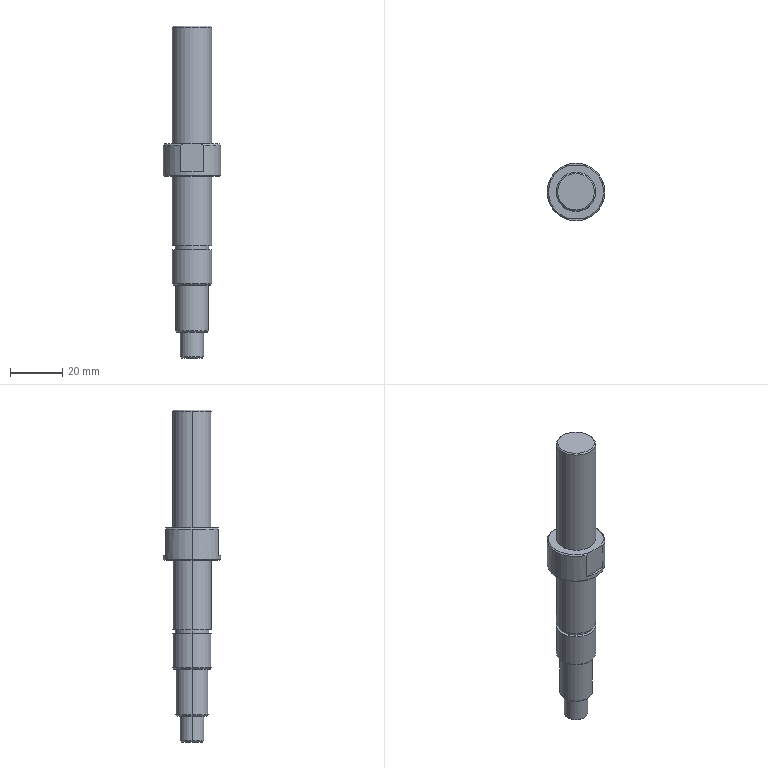Part | STEP file | 10000020499swp000-1 | 1 solid | 43 faces | box 22 x 22 x 126.85 mm | volume 22513 mm3 | cylinder 16 | cone 15 | plane 12 | commonest cylinder face diameters 15 x6 3.3 x2 9 x2 12.5 x2 12.8 x2 22 x2
STEP:
#1=CARTESIAN_POINT('',(7.5,0.,-84.));
#2=VERTEX_POINT('',#1);
#3=CARTESIAN_POINT('',(-7.5,0.,-84.));
#4=VERTEX_POINT('',#3);
#5=CARTESIAN_POINT('',(0.,0.,-84.));
#6=DIRECTION('',(0.,0.,1.));
#7=DIRECTION('',(1.,0.,0.));
#8=AXIS2_PLACEMENT_3D('',#5,#6,#7);
#9=CIRCLE('',#8,7.5);
#10=EDGE_CURVE('',#2,#4,#9,.T.);
#11=ORIENTED_EDGE('',*,*,#10,.T.);
#12=CARTESIAN_POINT('',(-7.5,0.,-57.5));
#13=VERTEX_POINT('',#12);
#14=CARTESIAN_POINT('',(-7.5,0.,-99.));
#15=DIRECTION('',(0.,0.,1.));
#16=VECTOR('',#15,1000.);
#17=LINE('',#14,#16);
#18=EDGE_CURVE('',#4,#13,#17,.T.);
#19=ORIENTED_EDGE('',*,*,#18,.T.);
#20=CARTESIAN_POINT('',(7.5,0.,-57.5));
#21=VERTEX_POINT('',#20);
#22=CARTESIAN_POINT('',(0.,0.,-57.5));
#23=DIRECTION('',(0.,0.,-1.));
#24=DIRECTION('',(-1.,0.,0.));
#25=AXIS2_PLACEMENT_3D('',#22,#23,#24);
#26=CIRCLE('',#25,7.5);
#27=EDGE_CURVE('',#13,#21,#26,.T.);
#28=ORIENTED_EDGE('',*,*,#27,.T.);
#29=CARTESIAN_POINT('',(7.5,0.,-99.));
#30=DIRECTION('',(0.,0.,1.));
#31=VECTOR('',#30,1000.);
#32=LINE('',#29,#31);
#33=EDGE_CURVE('',#2,#21,#32,.T.);
#34=ORIENTED_EDGE('',*,*,#33,.F.);
#35=EDGE_LOOP('',(#11,#19,#28,#34));
#36=FACE_OUTER_BOUND('',#35,.T.);
#37=CARTESIAN_POINT('',(0.,0.,-99.));
#38=DIRECTION('',(0.,0.,1.));
#39=DIRECTION('',(1.,0.,0.));
#40=AXIS2_PLACEMENT_3D('',#37,#38,#39);
#41=CYLINDRICAL_SURFACE('',#40,7.5);
#42=ADVANCED_FACE('',(#36),#41,.T.);
#43=CARTESIAN_POINT('',(-10.5,0.,-57.5));
#44=VERTEX_POINT('',#43);
#45=CARTESIAN_POINT('',(10.5,0.,-57.5));
#46=VERTEX_POINT('',#45);
#47=CARTESIAN_POINT('',(0.,0.,-57.5));
#48=DIRECTION('',(0.,0.,-1.));
#49=DIRECTION('',(-1.,0.,0.));
#50=AXIS2_PLACEMENT_3D('',#47,#48,#49);
#51=CIRCLE('',#50,10.5);
#52=EDGE_CURVE('',#44,#46,#51,.T.);
#53=ORIENTED_EDGE('',*,*,#52,.F.);
#54=CARTESIAN_POINT('',(-11.,0.,-57.));
#55=VERTEX_POINT('',#54);
#56=CARTESIAN_POINT('',(-10.5,0.,-57.5));
#57=DIRECTION('',(-0.7071,0.,0.7071));
#58=VECTOR('',#57,1000.);
#59=LINE('',#56,#58);
#60=EDGE_CURVE('',#44,#55,#59,.T.);
#61=ORIENTED_EDGE('',*,*,#60,.T.);
#62=CARTESIAN_POINT('',(11.,0.,-57.));
#63=VERTEX_POINT('',#62);
#64=CARTESIAN_POINT('',(0.,0.,-57.));
#65=DIRECTION('',(0.,0.,1.));
#66=DIRECTION('',(-1.,0.,0.));
#67=AXIS2_PLACEMENT_3D('',#64,#65,#66);
#68=CIRCLE('',#67,11.);
#69=EDGE_CURVE('',#63,#55,#68,.T.);
#70=ORIENTED_EDGE('',*,*,#69,.F.);
#71=CARTESIAN_POINT('',(10.5,0.,-57.5));
#72=DIRECTION('',(0.7071,0.,0.7071));
#73=VECTOR('',#72,1000.);
#74=LINE('',#71,#73);
#75=EDGE_CURVE('',#46,#63,#74,.T.);
#76=ORIENTED_EDGE('',*,*,#75,.F.);
#77=EDGE_LOOP('',(#53,#61,#70,#76));
#78=FACE_OUTER_BOUND('',#77,.T.);
#79=CARTESIAN_POINT('',(0.,0.,-57.5));
#80=DIRECTION('',(0.,0.,1.));
#81=DIRECTION('',(1.,0.,0.));
#82=AXIS2_PLACEMENT_3D('',#79,#80,#81);
#83=CONICAL_SURFACE('',#82,10.5,0.7854);
#84=ADVANCED_FACE('',(#78),#83,.T.);
#85=ORIENTED_EDGE('',*,*,#69,.T.);
#86=CARTESIAN_POINT('',(-11.,0.,-45.5));
#87=VERTEX_POINT('',#86);
#88=CARTESIAN_POINT('',(-11.,0.,-57.5));
#89=DIRECTION('',(0.,0.,1.));
#90=VECTOR('',#89,1000.);
#91=LINE('',#88,#90);
#92=EDGE_CURVE('',#55,#87,#91,.T.);
#93=ORIENTED_EDGE('',*,*,#92,.T.);
#94=CARTESIAN_POINT('',(-4.583,10.,-45.5));
#95=VERTEX_POINT('',#94);
#96=CARTESIAN_POINT('',(0.,0.,-45.5));
#97=DIRECTION('',(0.,0.,-1.));
#98=DIRECTION('',(-1.,0.,0.));
#99=AXIS2_PLACEMENT_3D('',#96,#97,#98);
#100=CIRCLE('',#99,11.);
#101=EDGE_CURVE('',#87,#95,#100,.T.);
#102=ORIENTED_EDGE('',*,*,#101,.T.);
#103=CARTESIAN_POINT('',(-4.583,10.,-55.5));
#104=VERTEX_POINT('',#103);
#105=CARTESIAN_POINT('',(-4.583,10.,-57.5));
#106=DIRECTION('',(0.,0.,1.));
#107=VECTOR('',#106,1000.);
#108=LINE('',#105,#107);
#109=EDGE_CURVE('',#104,#95,#108,.T.);
#110=ORIENTED_EDGE('',*,*,#109,.F.);
#111=CARTESIAN_POINT('',(4.583,10.,-55.5));
#112=VERTEX_POINT('',#111);
#113=CARTESIAN_POINT('',(0.,0.,-55.5));
#114=DIRECTION('',(0.,0.,1.));
#115=DIRECTION('',(1.,0.,0.));
#116=AXIS2_PLACEMENT_3D('',#113,#114,#115);
#117=CIRCLE('',#116,11.);
#118=EDGE_CURVE('',#112,#104,#117,.T.);
#119=ORIENTED_EDGE('',*,*,#118,.F.);
#120=CARTESIAN_POINT('',(4.583,10.,-45.5));
#121=VERTEX_POINT('',#120);
#122=CARTESIAN_POINT('',(4.583,10.,-57.5));
#123=DIRECTION('',(0.,0.,-1.));
#124=VECTOR('',#123,1000.);
#125=LINE('',#122,#124);
#126=EDGE_CURVE('',#121,#112,#125,.T.);
#127=ORIENTED_EDGE('',*,*,#126,.F.);
#128=CARTESIAN_POINT('',(11.,0.,-45.5));
#129=VERTEX_POINT('',#128);
#130=CARTESIAN_POINT('',(0.,0.,-45.5));
#131=DIRECTION('',(0.,0.,-1.));
#132=DIRECTION('',(-1.,0.,0.));
#133=AXIS2_PLACEMENT_3D('',#130,#131,#132);
#134=CIRCLE('',#133,11.);
#135=EDGE_CURVE('',#121,#129,#134,.T.);
#136=ORIENTED_EDGE('',*,*,#135,.T.);
#137=CARTESIAN_POINT('',(11.,0.,-57.5));
#138=DIRECTION('',(0.,0.,1.));
#139=VECTOR('',#138,1000.);
#140=LINE('',#137,#139);
#141=EDGE_CURVE('',#63,#129,#140,.T.);
#142=ORIENTED_EDGE('',*,*,#141,.F.);
#143=EDGE_LOOP('',(#85,#93,#102,#110,#119,#127,#136,#142));
#144=FACE_OUTER_BOUND('',#143,.T.);
#145=CARTESIAN_POINT('',(0.,0.,-57.5));
#146=DIRECTION('',(0.,0.,1.));
#147=DIRECTION('',(1.,0.,0.));
#148=AXIS2_PLACEMENT_3D('',#145,#146,#147);
#149=CYLINDRICAL_SURFACE('',#148,11.);
#150=ADVANCED_FACE('',(#144),#149,.T.);
#151=CARTESIAN_POINT('',(-10.5,0.,-45.));
#152=VERTEX_POINT('',#151);
#153=CARTESIAN_POINT('',(-3.202,-10.,-45.));
#154=VERTEX_POINT('',#153);
#155=CARTESIAN_POINT('',(0.,0.,-45.));
#156=DIRECTION('',(0.,0.,1.));
#157=DIRECTION('',(-1.,0.,0.));
#158=AXIS2_PLACEMENT_3D('',#155,#156,#157);
#159=CIRCLE('',#158,10.5);
#160=EDGE_CURVE('',#152,#154,#159,.T.);
#161=ORIENTED_EDGE('',*,*,#160,.F.);
#162=CARTESIAN_POINT('',(-11.,0.,-45.5));
#163=DIRECTION('',(-0.7071,0.,-0.7071));
#164=VECTOR('',#163,1000.);
#165=LINE('',#162,#164);
#166=EDGE_CURVE('',#152,#87,#165,.T.);
#167=ORIENTED_EDGE('',*,*,#166,.T.);
#168=CARTESIAN_POINT('',(-4.583,-10.,-45.5));
#169=VERTEX_POINT('',#168);
#170=CARTESIAN_POINT('',(0.,0.,-45.5));
#171=DIRECTION('',(0.,0.,-1.));
#172=DIRECTION('',(-1.,0.,0.));
#173=AXIS2_PLACEMENT_3D('',#170,#171,#172);
#174=CIRCLE('',#173,11.);
#175=EDGE_CURVE('',#169,#87,#174,.T.);
#176=ORIENTED_EDGE('',*,*,#175,.F.);
#177=CARTESIAN_POINT('',(-4.583,-10.,-45.5));
#178=CARTESIAN_POINT('',(-4.131,-10.,-45.312));
#179=CARTESIAN_POINT('',(-3.672,-10.,-45.143));
#180=CARTESIAN_POINT('',(-3.202,-10.,-45.));
#181=B_SPLINE_CURVE_WITH_KNOTS('',3,(#177,#178,#179,#180),.UNSPECIFIED.,.F.,.F.,(4,4),(0.02198,0.02345),.UNSPECIFIED.);
#182=EDGE_CURVE('',#169,#154,#181,.T.);
#183=ORIENTED_EDGE('',*,*,#182,.T.);
#184=EDGE_LOOP('',(#161,#167,#176,#183));
#185=FACE_OUTER_BOUND('',#184,.T.);
#186=CARTESIAN_POINT('',(0.,0.,-45.5));
#187=DIRECTION('',(0.,0.,-1.));
#188=DIRECTION('',(-1.,0.,0.));
#189=AXIS2_PLACEMENT_3D('',#186,#187,#188);
#190=CONICAL_SURFACE('',#189,11.,0.7854);
#191=ADVANCED_FACE('',(#185),#190,.T.);
#192=CARTESIAN_POINT('',(7.5,0.,-45.));
#193=VERTEX_POINT('',#192);
#194=CARTESIAN_POINT('',(-7.5,0.,-45.));
#195=VERTEX_POINT('',#194);
#196=CARTESIAN_POINT('',(0.,0.,-45.));
#197=DIRECTION('',(0.,0.,1.));
#198=DIRECTION('',(-1.,0.,0.));
#199=AXIS2_PLACEMENT_3D('',#196,#197,#198);
#200=CIRCLE('',#199,7.5);
#201=EDGE_CURVE('',#193,#195,#200,.T.);
#202=ORIENTED_EDGE('',*,*,#201,.T.);
#203=CARTESIAN_POINT('',(-7.5,0.,-0.5));
#204=VERTEX_POINT('',#203);
#205=CARTESIAN_POINT('',(-7.5,0.,-45.));
#206=DIRECTION('',(0.,0.,1.));
#207=VECTOR('',#206,1000.);
#208=LINE('',#205,#207);
#209=EDGE_CURVE('',#195,#204,#208,.T.);
#210=ORIENTED_EDGE('',*,*,#209,.T.);
#211=CARTESIAN_POINT('',(7.5,0.,-0.5));
#212=VERTEX_POINT('',#211);
#213=CARTESIAN_POINT('',(0.,0.,-0.5));
#214=DIRECTION('',(0.,0.,-1.));
#215=DIRECTION('',(1.,0.,0.));
#216=AXIS2_PLACEMENT_3D('',#213,#214,#215);
#217=CIRCLE('',#216,7.5);
#218=EDGE_CURVE('',#204,#212,#217,.T.);
#219=ORIENTED_EDGE('',*,*,#218,.T.);
#220=CARTESIAN_POINT('',(7.5,0.,-45.));
#221=DIRECTION('',(0.,0.,1.));
#222=VECTOR('',#221,1000.);
#223=LINE('',#220,#222);
#224=EDGE_CURVE('',#193,#212,#223,.T.);
#225=ORIENTED_EDGE('',*,*,#224,.F.);
#226=EDGE_LOOP('',(#202,#210,#219,#225));
#227=FACE_OUTER_BOUND('',#226,.T.);
#228=CARTESIAN_POINT('',(0.,0.,-45.));
#229=DIRECTION('',(0.,0.,1.));
#230=DIRECTION('',(1.,0.,0.));
#231=AXIS2_PLACEMENT_3D('',#228,#229,#230);
#232=CYLINDRICAL_SURFACE('',#231,7.5);
#233=ADVANCED_FACE('',(#227),#232,.T.);
#234=CARTESIAN_POINT('',(7.,0.,0.));
#235=VERTEX_POINT('',#234);
#236=CARTESIAN_POINT('',(-7.,0.,0.));
#237=VERTEX_POINT('',#236);
#238=CARTESIAN_POINT('',(0.,0.,0.));
#239=DIRECTION('',(0.,0.,1.));
#240=DIRECTION('',(1.,0.,0.));
#241=AXIS2_PLACEMENT_3D('',#238,#239,#240);
#242=CIRCLE('',#241,7.);
#243=EDGE_CURVE('',#235,#237,#242,.T.);
#244=ORIENTED_EDGE('',*,*,#243,.F.);
#245=CARTESIAN_POINT('',(7.,0.,0.));
#246=DIRECTION('',(0.7071,0.,-0.7071));
#247=VECTOR('',#246,1000.);
#248=LINE('',#245,#247);
#249=EDGE_CURVE('',#235,#212,#248,.T.);
#250=ORIENTED_EDGE('',*,*,#249,.T.);
#251=ORIENTED_EDGE('',*,*,#218,.F.);
#252=CARTESIAN_POINT('',(-7.,0.,0.));
#253=DIRECTION('',(-0.7071,0.,-0.7071));
#254=VECTOR('',#253,1000.);
#255=LINE('',#252,#254);
#256=EDGE_CURVE('',#237,#204,#255,.T.);
#257=ORIENTED_EDGE('',*,*,#256,.F.);
#258=EDGE_LOOP('',(#244,#250,#251,#257));
#259=FACE_OUTER_BOUND('',#258,.T.);
#260=CARTESIAN_POINT('',(0.,0.,0.));
#261=DIRECTION('',(0.,0.,-1.));
#262=DIRECTION('',(-1.,0.,0.));
#263=AXIS2_PLACEMENT_3D('',#260,#261,#262);
#264=CONICAL_SURFACE('',#263,7.,0.7854);
#265=ADVANCED_FACE('',(#259),#264,.T.);
#266=CARTESIAN_POINT('',(6.4,0.,-85.5));
#267=VERTEX_POINT('',#266);
#268=CARTESIAN_POINT('',(-6.4,0.,-85.5));
#269=VERTEX_POINT('',#268);
#270=CARTESIAN_POINT('',(0.,0.,-85.5));
#271=DIRECTION('',(0.,0.,1.));
#272=DIRECTION('',(1.,0.,0.));
#273=AXIS2_PLACEMENT_3D('',#270,#271,#272);
#274=CIRCLE('',#273,6.4);
#275=EDGE_CURVE('',#267,#269,#274,.T.);
#276=ORIENTED_EDGE('',*,*,#275,.T.);
#277=CARTESIAN_POINT('',(-6.4,0.,-84.));
#278=VERTEX_POINT('',#277);
#279=CARTESIAN_POINT('',(-6.4,0.,-126.85));
#280=DIRECTION('',(0.,0.,1.));
#281=VECTOR('',#280,1000.);
#282=LINE('',#279,#281);
#283=EDGE_CURVE('',#269,#278,#282,.T.);
#284=ORIENTED_EDGE('',*,*,#283,.T.);
#285=CARTESIAN_POINT('',(6.4,0.,-84.));
#286=VERTEX_POINT('',#285);
#287=CARTESIAN_POINT('',(0.,0.,-84.));
#288=DIRECTION('',(0.,0.,1.));
#289=DIRECTION('',(1.,0.,0.));
#290=AXIS2_PLACEMENT_3D('',#287,#288,#289);
#291=CIRCLE('',#290,6.4);
#292=EDGE_CURVE('',#286,#278,#291,.T.);
#293=ORIENTED_EDGE('',*,*,#292,.F.);
#294=CARTESIAN_POINT('',(6.4,0.,-126.85));
#295=DIRECTION('',(0.,0.,1.));
#296=VECTOR('',#295,1000.);
#297=LINE('',#294,#296);
#298=EDGE_CURVE('',#267,#286,#297,.T.);
#299=ORIENTED_EDGE('',*,*,#298,.F.);
#300=EDGE_LOOP('',(#276,#284,#293,#299));
#301=FACE_OUTER_BOUND('',#300,.T.);
#302=CARTESIAN_POINT('',(0.,0.,-126.85));
#303=DIRECTION('',(0.,0.,1.));
#304=DIRECTION('',(1.,0.,0.));
#305=AXIS2_PLACEMENT_3D('',#302,#303,#304);
#306=CYLINDRICAL_SURFACE('',#305,6.4);
#307=ADVANCED_FACE('',(#301),#306,.T.);
#308=CARTESIAN_POINT('',(1.65,0.,-112.75));
#309=VERTEX_POINT('',#308);
#310=CARTESIAN_POINT('',(-1.65,0.,-112.75));
#311=VERTEX_POINT('',#310);
#312=CARTESIAN_POINT('',(0.,0.,-112.75));
#313=DIRECTION('',(0.,0.,-1.));
#314=DIRECTION('',(-1.,0.,0.));
#315=AXIS2_PLACEMENT_3D('',#312,#313,#314);
#316=CIRCLE('',#315,1.65);
#317=EDGE_CURVE('',#309,#311,#316,.T.);
#318=ORIENTED_EDGE('',*,*,#317,.F.);
#319=CARTESIAN_POINT('',(1.65,0.,-126.85));
#320=VERTEX_POINT('',#319);
#321=CARTESIAN_POINT('',(1.65,0.,-126.85));
#322=DIRECTION('',(0.,0.,-1.));
#323=VECTOR('',#322,1000.);
#324=LINE('',#321,#323);
#325=EDGE_CURVE('',#309,#320,#324,.T.);
#326=ORIENTED_EDGE('',*,*,#325,.T.);
#327=CARTESIAN_POINT('',(-1.65,0.,-126.85));
#328=VERTEX_POINT('',#327);
#329=CARTESIAN_POINT('',(0.,0.,-126.85));
#330=DIRECTION('',(0.,0.,-1.));
#331=DIRECTION('',(-1.,0.,0.));
#332=AXIS2_PLACEMENT_3D('',#329,#330,#331);
#333=CIRCLE('',#332,1.65);
#334=EDGE_CURVE('',#320,#328,#333,.T.);
#335=ORIENTED_EDGE('',*,*,#334,.T.);
#336=CARTESIAN_POINT('',(-1.65,0.,-126.85));
#337=DIRECTION('',(0.,0.,-1.));
#338=VECTOR('',#337,1000.);
#339=LINE('',#336,#338);
#340=EDGE_CURVE('',#311,#328,#339,.T.);
#341=ORIENTED_EDGE('',*,*,#340,.F.);
#342=EDGE_LOOP('',(#318,#326,#335,#341));
#343=FACE_OUTER_BOUND('',#342,.T.);
#344=CARTESIAN_POINT('',(0.,0.,-126.85));
#345=DIRECTION('',(0.,0.,-1.));
#346=DIRECTION('',(-1.,0.,0.));
#347=AXIS2_PLACEMENT_3D('',#344,#345,#346);
#348=CYLINDRICAL_SURFACE('',#347,1.65);
#349=ADVANCED_FACE('',(#343),#348,.F.);
#350=CARTESIAN_POINT('',(0.,0.,-111.759));
#351=VERTEX_POINT('',#350);
#352=CARTESIAN_POINT('',(-1.65,0.,-112.75));
#353=DIRECTION('',(-0.8572,0.,-0.515));
#354=VECTOR('',#353,1000.);
#355=LINE('',#352,#354);
#356=EDGE_CURVE('',#351,#311,#355,.T.);
#357=ORIENTED_EDGE('',*,*,#356,.F.);
#358=CARTESIAN_POINT('',(1.65,0.,-112.75));
#359=DIRECTION('',(0.8572,0.,-0.515));
#360=VECTOR('',#359,1000.);
#361=LINE('',#358,#360);
#362=EDGE_CURVE('',#351,#309,#361,.T.);
#363=ORIENTED_EDGE('',*,*,#362,.T.);
#364=ORIENTED_EDGE('',*,*,#317,.T.);
#365=EDGE_LOOP('',(#357,#363,#364));
#366=FACE_OUTER_BOUND('',#365,.T.);
#367=CARTESIAN_POINT('',(0.,0.,-112.75));
#368=DIRECTION('',(0.,0.,-1.));
#369=DIRECTION('',(-1.,0.,0.));
#370=AXIS2_PLACEMENT_3D('',#367,#368,#369);
#371=CONICAL_SURFACE('',#370,1.65,1.03);
#372=ADVANCED_FACE('',(#366),#371,.F.);
#373=CARTESIAN_POINT('',(-4.,0.,-126.85));
#374=VERTEX_POINT('',#373);
#375=CARTESIAN_POINT('',(4.,0.,-126.85));
#376=VERTEX_POINT('',#375);
#377=CARTESIAN_POINT('',(0.,0.,-126.85));
#378=DIRECTION('',(0.,0.,-1.));
#379=DIRECTION('',(-1.,0.,0.));
#380=AXIS2_PLACEMENT_3D('',#377,#378,#379);
#381=CIRCLE('',#380,4.);
#382=EDGE_CURVE('',#374,#376,#381,.T.);
#383=ORIENTED_EDGE('',*,*,#382,.F.);
#384=CARTESIAN_POINT('',(-4.5,0.,-126.35));
#385=VERTEX_POINT('',#384);
#386=CARTESIAN_POINT('',(-4.,0.,-126.85));
#387=DIRECTION('',(-0.7071,0.,0.7071));
#388=VECTOR('',#387,1000.);
#389=LINE('',#386,#388);
#390=EDGE_CURVE('',#374,#385,#389,.T.);
#391=ORIENTED_EDGE('',*,*,#390,.T.);
#392=CARTESIAN_POINT('',(4.5,0.,-126.35));
#393=VERTEX_POINT('',#392);
#394=CARTESIAN_POINT('',(0.,0.,-126.35));
#395=DIRECTION('',(0.,0.,1.));
#396=DIRECTION('',(-1.,0.,0.));
#397=AXIS2_PLACEMENT_3D('',#394,#395,#396);
#398=CIRCLE('',#397,4.5);
#399=EDGE_CURVE('',#393,#385,#398,.T.);
#400=ORIENTED_EDGE('',*,*,#399,.F.);
#401=CARTESIAN_POINT('',(4.,0.,-126.85));
#402=DIRECTION('',(0.7071,0.,0.7071));
#403=VECTOR('',#402,1000.);
#404=LINE('',#401,#403);
#405=EDGE_CURVE('',#376,#393,#404,.T.);
#406=ORIENTED_EDGE('',*,*,#405,.F.);
#407=EDGE_LOOP('',(#383,#391,#400,#406));
#408=FACE_OUTER_BOUND('',#407,.T.);
#409=CARTESIAN_POINT('',(0.,0.,-126.85));
#410=DIRECTION('',(0.,0.,1.));
#411=DIRECTION('',(1.,0.,0.));
#412=AXIS2_PLACEMENT_3D('',#409,#410,#411);
#413=CONICAL_SURFACE('',#412,4.,0.7854);
#414=ADVANCED_FACE('',(#408),#413,.T.);
#415=CARTESIAN_POINT('',(-5.75,0.,-117.));
#416=VERTEX_POINT('',#415);
#417=CARTESIAN_POINT('',(5.75,0.,-117.));
#418=VERTEX_POINT('',#417);
#419=CARTESIAN_POINT('',(0.,0.,-117.));
#420=DIRECTION('',(0.,0.,-1.));
#421=DIRECTION('',(-1.,0.,0.));
#422=AXIS2_PLACEMENT_3D('',#419,#420,#421);
#423=CIRCLE('',#422,5.75);
#424=EDGE_CURVE('',#416,#418,#423,.T.);
#425=ORIENTED_EDGE('',*,*,#424,.F.);
#426=CARTESIAN_POINT('',(-6.25,0.,-116.5));
#427=VERTEX_POINT('',#426);
#428=CARTESIAN_POINT('',(-5.75,0.,-117.));
#429=DIRECTION('',(-0.7071,0.,0.7071));
#430=VECTOR('',#429,1000.);
#431=LINE('',#428,#430);
#432=EDGE_CURVE('',#416,#427,#431,.T.);
#433=ORIENTED_EDGE('',*,*,#432,.T.);
#434=CARTESIAN_POINT('',(6.25,0.,-116.5));
#435=VERTEX_POINT('',#434);
#436=CARTESIAN_POINT('',(0.,0.,-116.5));
#437=DIRECTION('',(0.,0.,1.));
#438=DIRECTION('',(-1.,0.,0.));
#439=AXIS2_PLACEMENT_3D('',#436,#437,#438);
#440=CIRCLE('',#439,6.25);
#441=EDGE_CURVE('',#435,#427,#440,.T.);
#442=ORIENTED_EDGE('',*,*,#441,.F.);
#443=CARTESIAN_POINT('',(5.75,0.,-117.));
#444=DIRECTION('',(0.7071,0.,0.7071));
#445=VECTOR('',#444,1000.);
#446=LINE('',#443,#445);
#447=EDGE_CURVE('',#418,#435,#446,.T.);
#448=ORIENTED_EDGE('',*,*,#447,.F.);
#449=EDGE_LOOP('',(#425,#433,#442,#448));
#450=FACE_OUTER_BOUND('',#449,.T.);
#451=CARTESIAN_POINT('',(0.,0.,-117.));
#452=DIRECTION('',(0.,0.,1.));
#453=DIRECTION('',(1.,0.,0.));
#454=AXIS2_PLACEMENT_3D('',#451,#452,#453);
#455=CONICAL_SURFACE('',#454,5.75,0.7854);
#456=ADVANCED_FACE('',(#450),#455,.T.);
#457=CARTESIAN_POINT('',(-7.,0.,-99.));
#458=VERTEX_POINT('',#457);
#459=CARTESIAN_POINT('',(7.,0.,-99.));
#460=VERTEX_POINT('',#459);
#461=CARTESIAN_POINT('',(0.,0.,-99.));
#462=DIRECTION('',(0.,0.,-1.));
#463=DIRECTION('',(-1.,0.,0.));
#464=AXIS2_PLACEMENT_3D('',#461,#462,#463);
#465=CIRCLE('',#464,7.);
#466=EDGE_CURVE('',#458,#460,#465,.T.);
#467=ORIENTED_EDGE('',*,*,#466,.F.);
#468=CARTESIAN_POINT('',(-7.5,0.,-98.5));
#469=VERTEX_POINT('',#468);
#470=CARTESIAN_POINT('',(-7.,0.,-99.));
#471=DIRECTION('',(-0.7071,0.,0.7071));
#472=VECTOR('',#471,1000.);
#473=LINE('',#470,#472);
#474=EDGE_CURVE('',#458,#469,#473,.T.);
#475=ORIENTED_EDGE('',*,*,#474,.T.);
#476=CARTESIAN_POINT('',(7.5,0.,-98.5));
#477=VERTEX_POINT('',#476);
#478=CARTESIAN_POINT('',(0.,0.,-98.5));
#479=DIRECTION('',(0.,0.,1.));
#480=DIRECTION('',(-1.,0.,0.));
#481=AXIS2_PLACEMENT_3D('',#478,#479,#480);
#482=CIRCLE('',#481,7.5);
#483=EDGE_CURVE('',#477,#469,#482,.T.);
#484=ORIENTED_EDGE('',*,*,#483,.F.);
#485=CARTESIAN_POINT('',(7.,0.,-99.));
#486=DIRECTION('',(0.7071,0.,0.7071));
#487=VECTOR('',#486,1000.);
#488=LINE('',#485,#487);
#489=EDGE_CURVE('',#460,#477,#488,.T.);
#490=ORIENTED_EDGE('',*,*,#489,.F.);
#491=EDGE_LOOP('',(#467,#475,#484,#490));
#492=FACE_OUTER_BOUND('',#491,.T.);
#493=CARTESIAN_POINT('',(0.,0.,-99.));
#494=DIRECTION('',(0.,0.,1.));
#495=DIRECTION('',(1.,0.,0.));
#496=AXIS2_PLACEMENT_3D('',#493,#494,#495);
#497=CONICAL_SURFACE('',#496,7.,0.7854);
#498=ADVANCED_FACE('',(#492),#497,.T.);
#499=ORIENTED_EDGE('',*,*,#399,.T.);
#500=CARTESIAN_POINT('',(-4.5,0.,-117.));
#501=VERTEX_POINT('',#500);
#502=CARTESIAN_POINT('',(-4.5,0.,-126.85));
#503=DIRECTION('',(0.,0.,1.));
#504=VECTOR('',#503,1000.);
#505=LINE('',#502,#504);
#506=EDGE_CURVE('',#385,#501,#505,.T.);
#507=ORIENTED_EDGE('',*,*,#506,.T.);
#508=CARTESIAN_POINT('',(4.5,0.,-117.));
#509=VERTEX_POINT('',#508);
#510=CARTESIAN_POINT('',(0.,0.,-117.));
#511=DIRECTION('',(0.,0.,-1.));
#512=DIRECTION('',(-1.,0.,0.));
#513=AXIS2_PLACEMENT_3D('',#510,#511,#512);
#514=CIRCLE('',#513,4.5);
#515=EDGE_CURVE('',#501,#509,#514,.T.);
#516=ORIENTED_EDGE('',*,*,#515,.T.);
#517=CARTESIAN_POINT('',(4.5,0.,-126.85));
#518=DIRECTION('',(0.,0.,1.));
#519=VECTOR('',#518,1000.);
#520=LINE('',#517,#519);
#521=EDGE_CURVE('',#393,#509,#520,.T.);
#522=ORIENTED_EDGE('',*,*,#521,.F.);
#523=EDGE_LOOP('',(#499,#507,#516,#522));
#524=FACE_OUTER_BOUND('',#523,.T.);
#525=CARTESIAN_POINT('',(0.,0.,-126.85));
#526=DIRECTION('',(0.,0.,1.));
#527=DIRECTION('',(1.,0.,0.));
#528=AXIS2_PLACEMENT_3D('',#525,#526,#527);
#529=CYLINDRICAL_SURFACE('',#528,4.5);
#530=ADVANCED_FACE('',(#524),#529,.T.);
#531=ORIENTED_EDGE('',*,*,#441,.T.);
#532=CARTESIAN_POINT('',(-6.25,0.,-99.));
#533=VERTEX_POINT('',#532);
#534=CARTESIAN_POINT('',(-6.25,0.,-117.));
#535=DIRECTION('',(0.,0.,1.));
#536=VECTOR('',#535,1000.);
#537=LINE('',#534,#536);
#538=EDGE_CURVE('',#427,#533,#537,.T.);
#539=ORIENTED_EDGE('',*,*,#538,.T.);
#540=CARTESIAN_POINT('',(6.25,0.,-99.));
#541=VERTEX_POINT('',#540);
#542=CARTESIAN_POINT('',(0.,0.,-99.));
#543=DIRECTION('',(0.,0.,-1.));
#544=DIRECTION('',(-1.,0.,0.));
#545=AXIS2_PLACEMENT_3D('',#542,#543,#544);
#546=CIRCLE('',#545,6.25);
#547=EDGE_CURVE('',#533,#541,#546,.T.);
#548=ORIENTED_EDGE('',*,*,#547,.T.);
#549=CARTESIAN_POINT('',(6.25,0.,-117.));
#550=DIRECTION('',(0.,0.,1.));
#551=VECTOR('',#550,1000.);
#552=LINE('',#549,#551);
#553=EDGE_CURVE('',#435,#541,#552,.T.);
#554=ORIENTED_EDGE('',*,*,#553,.F.);
#555=EDGE_LOOP('',(#531,#539,#548,#554));
#556=FACE_OUTER_BOUND('',#555,.T.);
#557=CARTESIAN_POINT('',(0.,0.,-117.));
#558=DIRECTION('',(0.,0.,1.));
#559=DIRECTION('',(1.,0.,0.));
#560=AXIS2_PLACEMENT_3D('',#557,#558,#559);
#561=CYLINDRICAL_SURFACE('',#560,6.25);
#562=ADVANCED_FACE('',(#556),#561,.T.);
#563=ORIENTED_EDGE('',*,*,#483,.T.);
#564=CARTESIAN_POINT('',(-7.5,0.,-85.5));
#565=VERTEX_POINT('',#564);
#566=CARTESIAN_POINT('',(-7.5,0.,-99.));
#567=DIRECTION('',(0.,0.,1.));
#568=VECTOR('',#567,1000.);
#569=LINE('',#566,#568);
#570=EDGE_CURVE('',#469,#565,#569,.T.);
#571=ORIENTED_EDGE('',*,*,#570,.T.);
#572=CARTESIAN_POINT('',(7.5,0.,-85.5));
#573=VERTEX_POINT('',#572);
#574=CARTESIAN_POINT('',(0.,0.,-85.5));
#575=DIRECTION('',(0.,0.,1.));
#576=DIRECTION('',(1.,0.,0.));
#577=AXIS2_PLACEMENT_3D('',#574,#575,#576);
#578=CIRCLE('',#577,7.5);
#579=EDGE_CURVE('',#573,#565,#578,.T.);
#580=ORIENTED_EDGE('',*,*,#579,.F.);
#581=CARTESIAN_POINT('',(7.5,0.,-99.));
#582=DIRECTION('',(0.,0.,1.));
#583=VECTOR('',#582,1000.);
#584=LINE('',#581,#583);
#585=EDGE_CURVE('',#477,#573,#584,.T.);
#586=ORIENTED_EDGE('',*,*,#585,.F.);
#587=EDGE_LOOP('',(#563,#571,#580,#586));
#588=FACE_OUTER_BOUND('',#587,.T.);
#589=CARTESIAN_POINT('',(0.,0.,-99.));
#590=DIRECTION('',(0.,0.,1.));
#591=DIRECTION('',(1.,0.,0.));
#592=AXIS2_PLACEMENT_3D('',#589,#590,#591);
#593=CYLINDRICAL_SURFACE('',#592,7.5);
#594=ADVANCED_FACE('',(#588),#593,.T.);
#595=ORIENTED_EDGE('',*,*,#570,.F.);
#596=CARTESIAN_POINT('',(0.,0.,-98.5));
#597=DIRECTION('',(0.,0.,1.));
#598=DIRECTION('',(-1.,0.,0.));
#599=AXIS2_PLACEMENT_3D('',#596,#597,#598);
#600=CIRCLE('',#599,7.5);
#601=EDGE_CURVE('',#469,#477,#600,.T.);
#602=ORIENTED_EDGE('',*,*,#601,.T.);
#603=ORIENTED_EDGE('',*,*,#585,.T.);
#604=CARTESIAN_POINT('',(0.,0.,-85.5));
#605=DIRECTION('',(0.,0.,1.));
#606=DIRECTION('',(1.,0.,0.));
#607=AXIS2_PLACEMENT_3D('',#604,#605,#606);
#608=CIRCLE('',#607,7.5);
#609=EDGE_CURVE('',#565,#573,#608,.T.);
#610=ORIENTED_EDGE('',*,*,#609,.F.);
#611=EDGE_LOOP('',(#595,#602,#603,#610));
#612=FACE_OUTER_BOUND('',#611,.T.);
#613=CARTESIAN_POINT('',(0.,0.,-99.));
#614=DIRECTION('',(0.,0.,1.));
#615=DIRECTION('',(1.,0.,0.));
#616=AXIS2_PLACEMENT_3D('',#613,#614,#615);
#617=CYLINDRICAL_SURFACE('',#616,7.5);
#618=ADVANCED_FACE('',(#612),#617,.T.);
#619=CARTESIAN_POINT('',(0.,0.,-99.));
#620=DIRECTION('',(0.,0.,-1.));
#621=DIRECTION('',(-1.,0.,0.));
#622=AXIS2_PLACEMENT_3D('',#619,#620,#621);
#623=CIRCLE('',#622,7.);
#624=EDGE_CURVE('',#460,#458,#623,.T.);
#625=ORIENTED_EDGE('',*,*,#624,.T.);
#626=ORIENTED_EDGE('',*,*,#466,.T.);
#627=EDGE_LOOP('',(#625,#626));
#628=FACE_OUTER_BOUND('',#627,.T.);
#629=CARTESIAN_POINT('',(0.,0.,-99.));
#630=DIRECTION('',(0.,0.,-1.));
#631=DIRECTION('',(-1.,0.,0.));
#632=AXIS2_PLACEMENT_3D('',#629,#630,#631);
#633=CIRCLE('',#632,6.25);
#634=EDGE_CURVE('',#541,#533,#633,.T.);
#635=ORIENTED_EDGE('',*,*,#634,.F.);
#636=ORIENTED_EDGE('',*,*,#547,.F.);
#637=EDGE_LOOP('',(#635,#636));
#638=FACE_BOUND('',#637,.T.);
#639=CARTESIAN_POINT('',(0.,0.,-99.));
#640=DIRECTION('',(0.,0.,-1.));
#641=DIRECTION('',(-1.,0.,0.));
#642=AXIS2_PLACEMENT_3D('',#639,#640,#641);
#643=PLANE('',#642);
#644=ADVANCED_FACE('',(#628,#638),#643,.T.);
#645=ORIENTED_EDGE('',*,*,#538,.F.);
#646=CARTESIAN_POINT('',(0.,0.,-116.5));
#647=DIRECTION('',(0.,0.,1.));
#648=DIRECTION('',(-1.,0.,0.));
#649=AXIS2_PLACEMENT_3D('',#646,#647,#648);
#650=CIRCLE('',#649,6.25);
#651=EDGE_CURVE('',#427,#435,#650,.T.);
#652=ORIENTED_EDGE('',*,*,#651,.T.);
#653=ORIENTED_EDGE('',*,*,#553,.T.);
#654=ORIENTED_EDGE('',*,*,#634,.T.);
#655=EDGE_LOOP('',(#645,#652,#653,#654));
#656=FACE_OUTER_BOUND('',#655,.T.);
#657=CARTESIAN_POINT('',(0.,0.,-117.));
#658=DIRECTION('',(0.,0.,1.));
#659=DIRECTION('',(1.,0.,0.));
#660=AXIS2_PLACEMENT_3D('',#657,#658,#659);
#661=CYLINDRICAL_SURFACE('',#660,6.25);
#662=ADVANCED_FACE('',(#656),#661,.T.);
#663=CARTESIAN_POINT('',(0.,0.,-117.));
#664=DIRECTION('',(0.,0.,-1.));
#665=DIRECTION('',(-1.,0.,0.));
#666=AXIS2_PLACEMENT_3D('',#663,#664,#665);
#667=CIRCLE('',#666,5.75);
#668=EDGE_CURVE('',#418,#416,#667,.T.);
#669=ORIENTED_EDGE('',*,*,#668,.T.);
#670=ORIENTED_EDGE('',*,*,#424,.T.);
#671=EDGE_LOOP('',(#669,#670));
#672=FACE_OUTER_BOUND('',#671,.T.);
#673=CARTESIAN_POINT('',(0.,0.,-117.));
#674=DIRECTION('',(0.,0.,-1.));
#675=DIRECTION('',(-1.,0.,0.));
#676=AXIS2_PLACEMENT_3D('',#673,#674,#675);
#677=CIRCLE('',#676,4.5);
#678=EDGE_CURVE('',#509,#501,#677,.T.);
#679=ORIENTED_EDGE('',*,*,#678,.F.);
#680=ORIENTED_EDGE('',*,*,#515,.F.);
#681=EDGE_LOOP('',(#679,#680));
#682=FACE_BOUND('',#681,.T.);
#683=CARTESIAN_POINT('',(0.,0.,-117.));
#684=DIRECTION('',(0.,0.,-1.));
#685=DIRECTION('',(-1.,0.,0.));
#686=AXIS2_PLACEMENT_3D('',#683,#684,#685);
#687=PLANE('',#686);
#688=ADVANCED_FACE('',(#672,#682),#687,.T.);
#689=ORIENTED_EDGE('',*,*,#506,.F.);
#690=CARTESIAN_POINT('',(0.,0.,-126.35));
#691=DIRECTION('',(0.,0.,1.));
#692=DIRECTION('',(-1.,0.,0.));
#693=AXIS2_PLACEMENT_3D('',#690,#691,#692);
#694=CIRCLE('',#693,4.5);
#695=EDGE_CURVE('',#385,#393,#694,.T.);
#696=ORIENTED_EDGE('',*,*,#695,.T.);
#697=ORIENTED_EDGE('',*,*,#521,.T.);
#698=ORIENTED_EDGE('',*,*,#678,.T.);
#699=EDGE_LOOP('',(#689,#696,#697,#698));
#700=FACE_OUTER_BOUND('',#699,.T.);
#701=CARTESIAN_POINT('',(0.,0.,-126.85));
#702=DIRECTION('',(0.,0.,1.));
#703=DIRECTION('',(1.,0.,0.));
#704=AXIS2_PLACEMENT_3D('',#701,#702,#703);
#705=CYLINDRICAL_SURFACE('',#704,4.5);
#706=ADVANCED_FACE('',(#700),#705,.T.);
#707=CARTESIAN_POINT('',(0.,0.,-126.85));
#708=DIRECTION('',(0.,0.,-1.));
#709=DIRECTION('',(-1.,0.,0.));
#710=AXIS2_PLACEMENT_3D('',#707,#708,#709);
#711=CIRCLE('',#710,1.65);
#712=EDGE_CURVE('',#328,#320,#711,.T.);
#713=ORIENTED_EDGE('',*,*,#712,.F.);
#714=ORIENTED_EDGE('',*,*,#334,.F.);
#715=EDGE_LOOP('',(#713,#714));
#716=FACE_BOUND('',#715,.T.);
#717=CARTESIAN_POINT('',(0.,0.,-126.85));
#718=DIRECTION('',(0.,0.,-1.));
#719=DIRECTION('',(-1.,0.,0.));
#720=AXIS2_PLACEMENT_3D('',#717,#718,#719);
#721=CIRCLE('',#720,4.);
#722=EDGE_CURVE('',#376,#374,#721,.T.);
#723=ORIENTED_EDGE('',*,*,#722,.T.);
#724=ORIENTED_EDGE('',*,*,#382,.T.);
#725=EDGE_LOOP('',(#723,#724));
#726=FACE_OUTER_BOUND('',#725,.T.);
#727=CARTESIAN_POINT('',(0.,0.,-126.85));
#728=DIRECTION('',(0.,0.,-1.));
#729=DIRECTION('',(-1.,0.,0.));
#730=AXIS2_PLACEMENT_3D('',#727,#728,#729);
#731=PLANE('',#730);
#732=ADVANCED_FACE('',(#716,#726),#731,.T.);
#733=ORIENTED_EDGE('',*,*,#474,.F.);
#734=ORIENTED_EDGE('',*,*,#624,.F.);
#735=ORIENTED_EDGE('',*,*,#489,.T.);
#736=ORIENTED_EDGE('',*,*,#601,.F.);
#737=EDGE_LOOP('',(#733,#734,#735,#736));
#738=FACE_OUTER_BOUND('',#737,.T.);
#739=CARTESIAN_POINT('',(0.,0.,-99.));
#740=DIRECTION('',(0.,0.,1.));
#741=DIRECTION('',(1.,0.,0.));
#742=AXIS2_PLACEMENT_3D('',#739,#740,#741);
#743=CONICAL_SURFACE('',#742,7.,0.7854);
#744=ADVANCED_FACE('',(#738),#743,.T.);
#745=ORIENTED_EDGE('',*,*,#432,.F.);
#746=ORIENTED_EDGE('',*,*,#668,.F.);
#747=ORIENTED_EDGE('',*,*,#447,.T.);
#748=ORIENTED_EDGE('',*,*,#651,.F.);
#749=EDGE_LOOP('',(#745,#746,#747,#748));
#750=FACE_OUTER_BOUND('',#749,.T.);
#751=CARTESIAN_POINT('',(0.,0.,-117.));
#752=DIRECTION('',(0.,0.,1.));
#753=DIRECTION('',(1.,0.,0.));
#754=AXIS2_PLACEMENT_3D('',#751,#752,#753);
#755=CONICAL_SURFACE('',#754,5.75,0.7854);
#756=ADVANCED_FACE('',(#750),#755,.T.);
#757=ORIENTED_EDGE('',*,*,#390,.F.);
#758=ORIENTED_EDGE('',*,*,#722,.F.);
#759=ORIENTED_EDGE('',*,*,#405,.T.);
#760=ORIENTED_EDGE('',*,*,#695,.F.);
#761=EDGE_LOOP('',(#757,#758,#759,#760));
#762=FACE_OUTER_BOUND('',#761,.T.);
#763=CARTESIAN_POINT('',(0.,0.,-126.85));
#764=DIRECTION('',(0.,0.,1.));
#765=DIRECTION('',(1.,0.,0.));
#766=AXIS2_PLACEMENT_3D('',#763,#764,#765);
#767=CONICAL_SURFACE('',#766,4.,0.7854);
#768=ADVANCED_FACE('',(#762),#767,.T.);
#769=ORIENTED_EDGE('',*,*,#362,.F.);
#770=ORIENTED_EDGE('',*,*,#356,.T.);
#771=CARTESIAN_POINT('',(0.,0.,-112.75));
#772=DIRECTION('',(0.,0.,-1.));
#773=DIRECTION('',(-1.,0.,0.));
#774=AXIS2_PLACEMENT_3D('',#771,#772,#773);
#775=CIRCLE('',#774,1.65);
#776=EDGE_CURVE('',#311,#309,#775,.T.);
#777=ORIENTED_EDGE('',*,*,#776,.T.);
#778=EDGE_LOOP('',(#769,#770,#777));
#779=FACE_OUTER_BOUND('',#778,.T.);
#780=CARTESIAN_POINT('',(0.,0.,-112.75));
#781=DIRECTION('',(0.,0.,-1.));
#782=DIRECTION('',(-1.,0.,0.));
#783=AXIS2_PLACEMENT_3D('',#780,#781,#782);
#784=CONICAL_SURFACE('',#783,1.65,1.03);
#785=ADVANCED_FACE('',(#779),#784,.F.);
#786=ORIENTED_EDGE('',*,*,#325,.F.);
#787=ORIENTED_EDGE('',*,*,#776,.F.);
#788=ORIENTED_EDGE('',*,*,#340,.T.);
#789=ORIENTED_EDGE('',*,*,#712,.T.);
#790=EDGE_LOOP('',(#786,#787,#788,#789));
#791=FACE_OUTER_BOUND('',#790,.T.);
#792=CARTESIAN_POINT('',(0.,0.,-126.85));
#793=DIRECTION('',(0.,0.,-1.));
#794=DIRECTION('',(-1.,0.,0.));
#795=AXIS2_PLACEMENT_3D('',#792,#793,#794);
#796=CYLINDRICAL_SURFACE('',#795,1.65);
#797=ADVANCED_FACE('',(#791),#796,.F.);
#798=ORIENTED_EDGE('',*,*,#579,.T.);
#799=ORIENTED_EDGE('',*,*,#609,.T.);
#800=EDGE_LOOP('',(#798,#799));
#801=FACE_OUTER_BOUND('',#800,.T.);
#802=ORIENTED_EDGE('',*,*,#275,.F.);
#803=CARTESIAN_POINT('',(0.,0.,-85.5));
#804=DIRECTION('',(0.,0.,1.));
#805=DIRECTION('',(1.,0.,0.));
#806=AXIS2_PLACEMENT_3D('',#803,#804,#805);
#807=CIRCLE('',#806,6.4);
#808=EDGE_CURVE('',#269,#267,#807,.T.);
#809=ORIENTED_EDGE('',*,*,#808,.F.);
#810=EDGE_LOOP('',(#802,#809));
#811=FACE_BOUND('',#810,.T.);
#812=CARTESIAN_POINT('',(0.,7.5,-85.5));
#813=DIRECTION('',(0.,0.,1.));
#814=DIRECTION('',(1.,0.,0.));
#815=AXIS2_PLACEMENT_3D('',#812,#813,#814);
#816=PLANE('',#815);
#817=ADVANCED_FACE('',(#801,#811),#816,.T.);
#818=ORIENTED_EDGE('',*,*,#283,.F.);
#819=ORIENTED_EDGE('',*,*,#808,.T.);
#820=ORIENTED_EDGE('',*,*,#298,.T.);
#821=CARTESIAN_POINT('',(0.,0.,-84.));
#822=DIRECTION('',(0.,0.,1.));
#823=DIRECTION('',(1.,0.,0.));
#824=AXIS2_PLACEMENT_3D('',#821,#822,#823);
#825=CIRCLE('',#824,6.4);
#826=EDGE_CURVE('',#278,#286,#825,.T.);
#827=ORIENTED_EDGE('',*,*,#826,.F.);
#828=EDGE_LOOP('',(#818,#819,#820,#827));
#829=FACE_OUTER_BOUND('',#828,.T.);
#830=CARTESIAN_POINT('',(0.,0.,-126.85));
#831=DIRECTION('',(0.,0.,1.));
#832=DIRECTION('',(1.,0.,0.));
#833=AXIS2_PLACEMENT_3D('',#830,#831,#832);
#834=CYLINDRICAL_SURFACE('',#833,6.4);
#835=ADVANCED_FACE('',(#829),#834,.T.);
#836=ORIENTED_EDGE('',*,*,#292,.T.);
#837=ORIENTED_EDGE('',*,*,#826,.T.);
#838=EDGE_LOOP('',(#836,#837));
#839=FACE_BOUND('',#838,.T.);
#840=ORIENTED_EDGE('',*,*,#10,.F.);
#841=CARTESIAN_POINT('',(0.,0.,-84.));
#842=DIRECTION('',(0.,0.,1.));
#843=DIRECTION('',(1.,0.,0.));
#844=AXIS2_PLACEMENT_3D('',#841,#842,#843);
#845=CIRCLE('',#844,7.5);
#846=EDGE_CURVE('',#4,#2,#845,.T.);
#847=ORIENTED_EDGE('',*,*,#846,.F.);
#848=EDGE_LOOP('',(#840,#847));
#849=FACE_OUTER_BOUND('',#848,.T.);
#850=CARTESIAN_POINT('',(0.,7.5,-84.));
#851=DIRECTION('',(0.,0.,-1.));
#852=DIRECTION('',(-1.,0.,0.));
#853=AXIS2_PLACEMENT_3D('',#850,#851,#852);
#854=PLANE('',#853);
#855=ADVANCED_FACE('',(#839,#849),#854,.T.);
#856=CARTESIAN_POINT('',(0.,0.,0.));
#857=DIRECTION('',(0.,0.,1.));
#858=DIRECTION('',(1.,0.,0.));
#859=AXIS2_PLACEMENT_3D('',#856,#857,#858);
#860=CIRCLE('',#859,7.);
#861=EDGE_CURVE('',#237,#235,#860,.T.);
#862=ORIENTED_EDGE('',*,*,#861,.T.);
#863=ORIENTED_EDGE('',*,*,#243,.T.);
#864=EDGE_LOOP('',(#862,#863));
#865=FACE_OUTER_BOUND('',#864,.T.);
#866=CARTESIAN_POINT('',(0.,0.,0.));
#867=DIRECTION('',(0.,0.,1.));
#868=DIRECTION('',(1.,0.,0.));
#869=AXIS2_PLACEMENT_3D('',#866,#867,#868);
#870=PLANE('',#869);
#871=ADVANCED_FACE('',(#865),#870,.T.);
#872=ORIENTED_EDGE('',*,*,#249,.F.);
#873=ORIENTED_EDGE('',*,*,#861,.F.);
#874=ORIENTED_EDGE('',*,*,#256,.T.);
#875=CARTESIAN_POINT('',(0.,0.,-0.5));
#876=DIRECTION('',(0.,0.,-1.));
#877=DIRECTION('',(1.,0.,0.));
#878=AXIS2_PLACEMENT_3D('',#875,#876,#877);
#879=CIRCLE('',#878,7.5);
#880=EDGE_CURVE('',#212,#204,#879,.T.);
#881=ORIENTED_EDGE('',*,*,#880,.F.);
#882=EDGE_LOOP('',(#872,#873,#874,#881));
#883=FACE_OUTER_BOUND('',#882,.T.);
#884=CARTESIAN_POINT('',(0.,0.,0.));
#885=DIRECTION('',(0.,0.,-1.));
#886=DIRECTION('',(-1.,0.,0.));
#887=AXIS2_PLACEMENT_3D('',#884,#885,#886);
#888=CONICAL_SURFACE('',#887,7.,0.7854);
#889=ADVANCED_FACE('',(#883),#888,.T.);
#890=ORIENTED_EDGE('',*,*,#209,.F.);
#891=CARTESIAN_POINT('',(0.,0.,-45.));
#892=DIRECTION('',(0.,0.,1.));
#893=DIRECTION('',(-1.,0.,0.));
#894=AXIS2_PLACEMENT_3D('',#891,#892,#893);
#895=CIRCLE('',#894,7.5);
#896=EDGE_CURVE('',#195,#193,#895,.T.);
#897=ORIENTED_EDGE('',*,*,#896,.T.);
#898=ORIENTED_EDGE('',*,*,#224,.T.);
#899=ORIENTED_EDGE('',*,*,#880,.T.);
#900=EDGE_LOOP('',(#890,#897,#898,#899));
#901=FACE_OUTER_BOUND('',#900,.T.);
#902=CARTESIAN_POINT('',(0.,0.,-45.));
#903=DIRECTION('',(0.,0.,1.));
#904=DIRECTION('',(1.,0.,0.));
#905=AXIS2_PLACEMENT_3D('',#902,#903,#904);
#906=CYLINDRICAL_SURFACE('',#905,7.5);
#907=ADVANCED_FACE('',(#901),#906,.T.);
#908=ORIENTED_EDGE('',*,*,#201,.F.);
#909=ORIENTED_EDGE('',*,*,#896,.F.);
#910=EDGE_LOOP('',(#908,#909));
#911=FACE_BOUND('',#910,.T.);
#912=CARTESIAN_POINT('',(3.202,-10.,-45.));
#913=VERTEX_POINT('',#912);
#914=CARTESIAN_POINT('',(-12.263,-10.,-45.));
#915=DIRECTION('',(1.,0.,0.));
#916=VECTOR('',#915,1000.);
#917=LINE('',#914,#916);
#918=EDGE_CURVE('',#154,#913,#917,.T.);
#919=ORIENTED_EDGE('',*,*,#918,.T.);
#920=CARTESIAN_POINT('',(3.202,10.,-45.));
#921=VERTEX_POINT('',#920);
#922=CARTESIAN_POINT('',(0.,0.,-45.));
#923=DIRECTION('',(0.,0.,1.));
#924=DIRECTION('',(-1.,0.,0.));
#925=AXIS2_PLACEMENT_3D('',#922,#923,#924);
#926=CIRCLE('',#925,10.5);
#927=EDGE_CURVE('',#913,#921,#926,.T.);
#928=ORIENTED_EDGE('',*,*,#927,.T.);
#929=CARTESIAN_POINT('',(-3.202,10.,-45.));
#930=VERTEX_POINT('',#929);
#931=CARTESIAN_POINT('',(-12.263,10.,-45.));
#932=DIRECTION('',(1.,0.,0.));
#933=VECTOR('',#932,1000.);
#934=LINE('',#931,#933);
#935=EDGE_CURVE('',#930,#921,#934,.T.);
#936=ORIENTED_EDGE('',*,*,#935,.F.);
#937=CARTESIAN_POINT('',(0.,0.,-45.));
#938=DIRECTION('',(0.,0.,1.));
#939=DIRECTION('',(-1.,0.,0.));
#940=AXIS2_PLACEMENT_3D('',#937,#938,#939);
#941=CIRCLE('',#940,10.5);
#942=EDGE_CURVE('',#930,#152,#941,.T.);
#943=ORIENTED_EDGE('',*,*,#942,.T.);
#944=ORIENTED_EDGE('',*,*,#160,.T.);
#945=EDGE_LOOP('',(#919,#928,#936,#943,#944));
#946=FACE_OUTER_BOUND('',#945,.T.);
#947=CARTESIAN_POINT('',(0.,0.,-45.));
#948=DIRECTION('',(0.,0.,-1.));
#949=DIRECTION('',(-1.,0.,0.));
#950=AXIS2_PLACEMENT_3D('',#947,#948,#949);
#951=PLANE('',#950);
#952=ADVANCED_FACE('',(#911,#946),#951,.F.);
#953=ORIENTED_EDGE('',*,*,#927,.F.);
#954=CARTESIAN_POINT('',(4.583,-10.,-45.5));
#955=VERTEX_POINT('',#954);
#956=CARTESIAN_POINT('',(3.202,-10.,-45.));
#957=CARTESIAN_POINT('',(3.668,-10.,-45.142));
#958=CARTESIAN_POINT('',(4.131,-10.,-45.312));
#959=CARTESIAN_POINT('',(4.583,-10.,-45.5));
#960=B_SPLINE_CURVE_WITH_KNOTS('',3,(#956,#957,#958,#959),.UNSPECIFIED.,.F.,.F.,(4,4),(0.02995,0.03141),.UNSPECIFIED.);
#961=EDGE_CURVE('',#913,#955,#960,.T.);
#962=ORIENTED_EDGE('',*,*,#961,.T.);
#963=CARTESIAN_POINT('',(0.,0.,-45.5));
#964=DIRECTION('',(0.,0.,-1.));
#965=DIRECTION('',(-1.,0.,0.));
#966=AXIS2_PLACEMENT_3D('',#963,#964,#965);
#967=CIRCLE('',#966,11.);
#968=EDGE_CURVE('',#129,#955,#967,.T.);
#969=ORIENTED_EDGE('',*,*,#968,.F.);
#970=ORIENTED_EDGE('',*,*,#135,.F.);
#971=CARTESIAN_POINT('',(4.583,10.,-45.5));
#972=CARTESIAN_POINT('',(4.131,10.,-45.312));
#973=CARTESIAN_POINT('',(3.672,10.,-45.143));
#974=CARTESIAN_POINT('',(3.202,10.,-45.));
#975=B_SPLINE_CURVE_WITH_KNOTS('',3,(#971,#972,#973,#974),.UNSPECIFIED.,.F.,.F.,(4,4),(0.02198,0.02345),.UNSPECIFIED.);
#976=EDGE_CURVE('',#121,#921,#975,.T.);
#977=ORIENTED_EDGE('',*,*,#976,.T.);
#978=EDGE_LOOP('',(#953,#962,#969,#970,#977));
#979=FACE_OUTER_BOUND('',#978,.T.);
#980=CARTESIAN_POINT('',(0.,0.,-45.5));
#981=DIRECTION('',(0.,0.,-1.));
#982=DIRECTION('',(-1.,0.,0.));
#983=AXIS2_PLACEMENT_3D('',#980,#981,#982);
#984=CONICAL_SURFACE('',#983,11.,0.7854);
#985=ADVANCED_FACE('',(#979),#984,.T.);
#986=ORIENTED_EDGE('',*,*,#118,.T.);
#987=CARTESIAN_POINT('',(-12.263,10.,-55.5));
#988=DIRECTION('',(-1.,0.,0.));
#989=VECTOR('',#988,1000.);
#990=LINE('',#987,#989);
#991=EDGE_CURVE('',#112,#104,#990,.T.);
#992=ORIENTED_EDGE('',*,*,#991,.F.);
#993=EDGE_LOOP('',(#986,#992));
#994=FACE_OUTER_BOUND('',#993,.T.);
#995=CARTESIAN_POINT('',(-12.263,19.85,-55.5));
#996=DIRECTION('',(0.,0.,1.));
#997=DIRECTION('',(1.,0.,0.));
#998=AXIS2_PLACEMENT_3D('',#995,#996,#997);
#999=PLANE('',#998);
#1000=ADVANCED_FACE('',(#994),#999,.T.);
#1001=ORIENTED_EDGE('',*,*,#126,.T.);
#1002=ORIENTED_EDGE('',*,*,#991,.T.);
#1003=ORIENTED_EDGE('',*,*,#109,.T.);
#1004=CARTESIAN_POINT('',(-3.202,10.,-45.));
#1005=CARTESIAN_POINT('',(-3.668,10.,-45.142));
#1006=CARTESIAN_POINT('',(-4.131,10.,-45.312));
#1007=CARTESIAN_POINT('',(-4.583,10.,-45.5));
#1008=B_SPLINE_CURVE_WITH_KNOTS('',3,(#1004,#1005,#1006,#1007),.UNSPECIFIED.,.F.,.F.,(4,4),(0.02995,0.03141),.UNSPECIFIED.);
#1009=EDGE_CURVE('',#930,#95,#1008,.T.);
#1010=ORIENTED_EDGE('',*,*,#1009,.F.);
#1011=ORIENTED_EDGE('',*,*,#935,.T.);
#1012=ORIENTED_EDGE('',*,*,#976,.F.);
#1013=EDGE_LOOP('',(#1001,#1002,#1003,#1010,#1011,#1012));
#1014=FACE_OUTER_BOUND('',#1013,.T.);
#1015=CARTESIAN_POINT('',(0.,10.,0.));
#1016=DIRECTION('',(0.,1.,0.));
#1017=DIRECTION('',(0.,0.,1.));
#1018=AXIS2_PLACEMENT_3D('',#1015,#1016,#1017);
#1019=PLANE('',#1018);
#1020=ADVANCED_FACE('',(#1014),#1019,.T.);
#1021=ORIENTED_EDGE('',*,*,#166,.F.);
#1022=ORIENTED_EDGE('',*,*,#942,.F.);
#1023=ORIENTED_EDGE('',*,*,#1009,.T.);
#1024=ORIENTED_EDGE('',*,*,#101,.F.);
#1025=EDGE_LOOP('',(#1021,#1022,#1023,#1024));
#1026=FACE_OUTER_BOUND('',#1025,.T.);
#1027=CARTESIAN_POINT('',(0.,0.,-45.5));
#1028=DIRECTION('',(0.,0.,-1.));
#1029=DIRECTION('',(-1.,0.,0.));
#1030=AXIS2_PLACEMENT_3D('',#1027,#1028,#1029);
#1031=CONICAL_SURFACE('',#1030,11.,0.7854);
#1032=ADVANCED_FACE('',(#1026),#1031,.T.);
#1033=CARTESIAN_POINT('',(4.583,-10.,-55.5));
#1034=VERTEX_POINT('',#1033);
#1035=CARTESIAN_POINT('',(-4.583,-10.,-55.5));
#1036=VERTEX_POINT('',#1035);
#1037=CARTESIAN_POINT('',(-12.263,-10.,-55.5));
#1038=DIRECTION('',(-1.,0.,0.));
#1039=VECTOR('',#1038,1000.);
#1040=LINE('',#1037,#1039);
#1041=EDGE_CURVE('',#1034,#1036,#1040,.T.);
#1042=ORIENTED_EDGE('',*,*,#1041,.T.);
#1043=CARTESIAN_POINT('',(0.,0.,-55.5));
#1044=DIRECTION('',(0.,0.,-1.));
#1045=DIRECTION('',(-1.,0.,0.));
#1046=AXIS2_PLACEMENT_3D('',#1043,#1044,#1045);
#1047=CIRCLE('',#1046,11.);
#1048=EDGE_CURVE('',#1034,#1036,#1047,.T.);
#1049=ORIENTED_EDGE('',*,*,#1048,.F.);
#1050=EDGE_LOOP('',(#1042,#1049));
#1051=FACE_OUTER_BOUND('',#1050,.T.);
#1052=CARTESIAN_POINT('',(-12.263,-19.85,-55.5));
#1053=DIRECTION('',(0.,0.,-1.));
#1054=DIRECTION('',(-1.,0.,0.));
#1055=AXIS2_PLACEMENT_3D('',#1052,#1053,#1054);
#1056=PLANE('',#1055);
#1057=ADVANCED_FACE('',(#1051),#1056,.F.);
#1058=CARTESIAN_POINT('',(-4.583,-10.,-57.5));
#1059=DIRECTION('',(0.,0.,-1.));
#1060=VECTOR('',#1059,1000.);
#1061=LINE('',#1058,#1060);
#1062=EDGE_CURVE('',#169,#1036,#1061,.T.);
#1063=ORIENTED_EDGE('',*,*,#1062,.T.);
#1064=ORIENTED_EDGE('',*,*,#1041,.F.);
#1065=CARTESIAN_POINT('',(4.583,-10.,-57.5));
#1066=DIRECTION('',(0.,0.,1.));
#1067=VECTOR('',#1066,1000.);
#1068=LINE('',#1065,#1067);
#1069=EDGE_CURVE('',#1034,#955,#1068,.T.);
#1070=ORIENTED_EDGE('',*,*,#1069,.T.);
#1071=ORIENTED_EDGE('',*,*,#961,.F.);
#1072=ORIENTED_EDGE('',*,*,#918,.F.);
#1073=ORIENTED_EDGE('',*,*,#182,.F.);
#1074=EDGE_LOOP('',(#1063,#1064,#1070,#1071,#1072,#1073));
#1075=FACE_OUTER_BOUND('',#1074,.T.);
#1076=CARTESIAN_POINT('',(0.,-10.,0.));
#1077=DIRECTION('',(0.,-1.,0.));
#1078=DIRECTION('',(0.,0.,1.));
#1079=AXIS2_PLACEMENT_3D('',#1076,#1077,#1078);
#1080=PLANE('',#1079);
#1081=ADVANCED_FACE('',(#1075),#1080,.T.);
#1082=ORIENTED_EDGE('',*,*,#92,.F.);
#1083=CARTESIAN_POINT('',(0.,0.,-57.));
#1084=DIRECTION('',(0.,0.,1.));
#1085=DIRECTION('',(-1.,0.,0.));
#1086=AXIS2_PLACEMENT_3D('',#1083,#1084,#1085);
#1087=CIRCLE('',#1086,11.);
#1088=EDGE_CURVE('',#55,#63,#1087,.T.);
#1089=ORIENTED_EDGE('',*,*,#1088,.T.);
#1090=ORIENTED_EDGE('',*,*,#141,.T.);
#1091=ORIENTED_EDGE('',*,*,#968,.T.);
#1092=ORIENTED_EDGE('',*,*,#1069,.F.);
#1093=ORIENTED_EDGE('',*,*,#1048,.T.);
#1094=ORIENTED_EDGE('',*,*,#1062,.F.);
#1095=ORIENTED_EDGE('',*,*,#175,.T.);
#1096=EDGE_LOOP('',(#1082,#1089,#1090,#1091,#1092,#1093,#1094,#1095));
#1097=FACE_OUTER_BOUND('',#1096,.T.);
#1098=CARTESIAN_POINT('',(0.,0.,-57.5));
#1099=DIRECTION('',(0.,0.,1.));
#1100=DIRECTION('',(1.,0.,0.));
#1101=AXIS2_PLACEMENT_3D('',#1098,#1099,#1100);
#1102=CYLINDRICAL_SURFACE('',#1101,11.);
#1103=ADVANCED_FACE('',(#1097),#1102,.T.);
#1104=ORIENTED_EDGE('',*,*,#60,.F.);
#1105=CARTESIAN_POINT('',(0.,0.,-57.5));
#1106=DIRECTION('',(0.,0.,-1.));
#1107=DIRECTION('',(-1.,0.,0.));
#1108=AXIS2_PLACEMENT_3D('',#1105,#1106,#1107);
#1109=CIRCLE('',#1108,10.5);
#1110=EDGE_CURVE('',#46,#44,#1109,.T.);
#1111=ORIENTED_EDGE('',*,*,#1110,.F.);
#1112=ORIENTED_EDGE('',*,*,#75,.T.);
#1113=ORIENTED_EDGE('',*,*,#1088,.F.);
#1114=EDGE_LOOP('',(#1104,#1111,#1112,#1113));
#1115=FACE_OUTER_BOUND('',#1114,.T.);
#1116=CARTESIAN_POINT('',(0.,0.,-57.5));
#1117=DIRECTION('',(0.,0.,1.));
#1118=DIRECTION('',(1.,0.,0.));
#1119=AXIS2_PLACEMENT_3D('',#1116,#1117,#1118);
#1120=CONICAL_SURFACE('',#1119,10.5,0.7854);
#1121=ADVANCED_FACE('',(#1115),#1120,.T.);
#1122=ORIENTED_EDGE('',*,*,#1110,.T.);
#1123=ORIENTED_EDGE('',*,*,#52,.T.);
#1124=EDGE_LOOP('',(#1122,#1123));
#1125=FACE_OUTER_BOUND('',#1124,.T.);
#1126=CARTESIAN_POINT('',(0.,0.,-57.5));
#1127=DIRECTION('',(0.,0.,-1.));
#1128=DIRECTION('',(-1.,0.,0.));
#1129=AXIS2_PLACEMENT_3D('',#1126,#1127,#1128);
#1130=CIRCLE('',#1129,7.5);
#1131=EDGE_CURVE('',#21,#13,#1130,.T.);
#1132=ORIENTED_EDGE('',*,*,#1131,.F.);
#1133=ORIENTED_EDGE('',*,*,#27,.F.);
#1134=EDGE_LOOP('',(#1132,#1133));
#1135=FACE_BOUND('',#1134,.T.);
#1136=CARTESIAN_POINT('',(0.,0.,-57.5));
#1137=DIRECTION('',(0.,0.,-1.));
#1138=DIRECTION('',(-1.,0.,0.));
#1139=AXIS2_PLACEMENT_3D('',#1136,#1137,#1138);
#1140=PLANE('',#1139);
#1141=ADVANCED_FACE('',(#1125,#1135),#1140,.T.);
#1142=ORIENTED_EDGE('',*,*,#18,.F.);
#1143=ORIENTED_EDGE('',*,*,#846,.T.);
#1144=ORIENTED_EDGE('',*,*,#33,.T.);
#1145=ORIENTED_EDGE('',*,*,#1131,.T.);
#1146=EDGE_LOOP('',(#1142,#1143,#1144,#1145));
#1147=FACE_OUTER_BOUND('',#1146,.T.);
#1148=CARTESIAN_POINT('',(0.,0.,-99.));
#1149=DIRECTION('',(0.,0.,1.));
#1150=DIRECTION('',(1.,0.,0.));
#1151=AXIS2_PLACEMENT_3D('',#1148,#1149,#1150);
#1152=CYLINDRICAL_SURFACE('',#1151,7.5);
#1153=ADVANCED_FACE('',(#1147),#1152,.T.);
#1154=CLOSED_SHELL('',(#42,#84,#150,#191,#233,#265,#307,#349,#372,#414,#456,#498,#530,#562,#594,#618,#644,#662,#688,#706,#732,#744,#756,#768,#785,#797,#817,#835,#855,#871,#889,#907,#952,#985,#1000,#1020,#1032,#1057,#1081,#1103,#1121,#1141,#1153));
#1155=MANIFOLD_SOLID_BREP('',#1154);
#1156=CARTESIAN_POINT('',(0.,0.,0.));
#1157=DIRECTION('',(0.,0.,1.));
#1158=DIRECTION('',(1.,0.,0.));
#1159=AXIS2_PLACEMENT_3D('',#1156,#1157,#1158);
#1160=(LENGTH_UNIT()NAMED_UNIT(*)SI_UNIT(.MILLI.,.METRE.));
#1161=UNCERTAINTY_MEASURE_WITH_UNIT(LENGTH_MEASURE(0.00001),#1160,'','');
#1162=(NAMED_UNIT(*)PLANE_ANGLE_UNIT()SI_UNIT($,.RADIAN.));
#1163=(NAMED_UNIT(*)SI_UNIT($,.STERADIAN.)SOLID_ANGLE_UNIT());
#1164=(GEOMETRIC_REPRESENTATION_CONTEXT(3)GLOBAL_UNCERTAINTY_ASSIGNED_CONTEXT((#1161))GLOBAL_UNIT_ASSIGNED_CONTEXT((#1160,#1162,#1163))REPRESENTATION_CONTEXT('',''));
#1165=ADVANCED_BREP_SHAPE_REPRESENTATION('',(#1155,#1159),#1164);